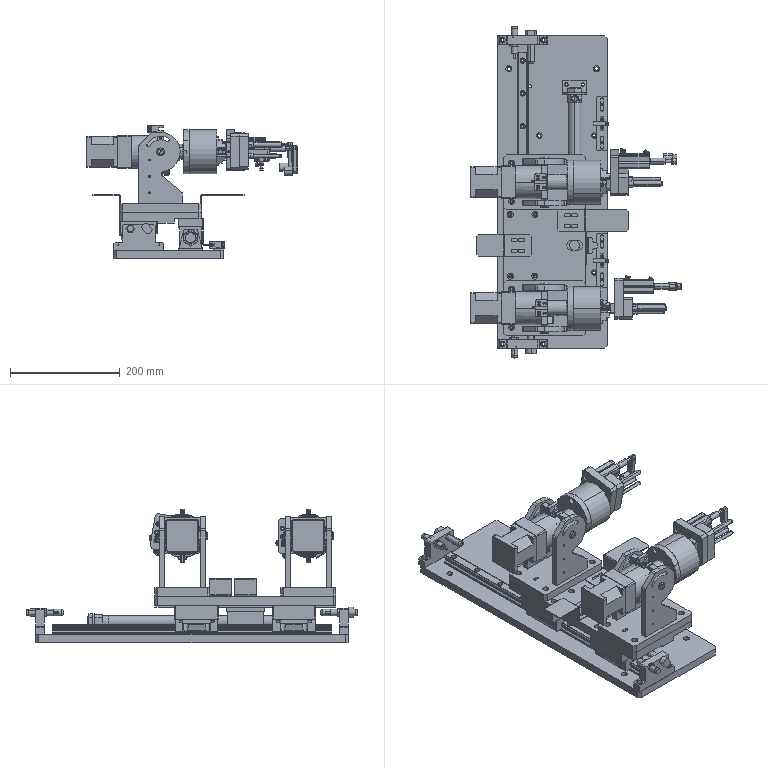Part | SolidWorks | 100 solids | 4280 faces | volume 5934131 mm3 | plane 1904 | cylinder 1794 | cone 494 | spline 52 | torus 24 | sphere 12 | commonest cylinder face diameters 5 x140 10 x122 3.3 x116 8 x108 6.6 x100 11 x100